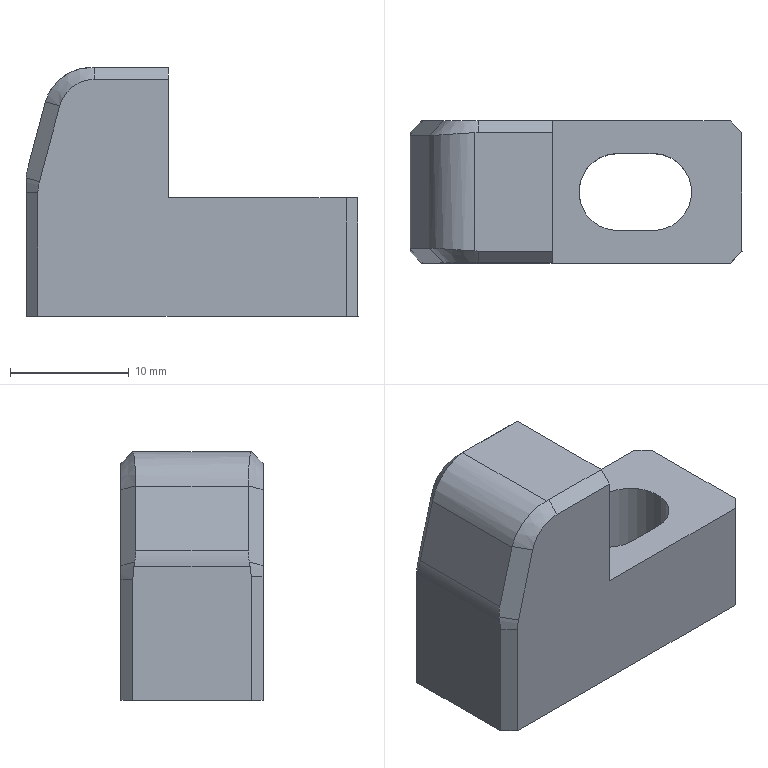Part | STEP file | gslz 2016.10.28-6_id682_x_t | 1 solid | 27 faces | box 28.004 x 12 x 21.002 mm | volume 4222 mm3 | plane 19 | cylinder 4 | cone 4 | commonest cylinder face diameters 6.5 x2 8 x1 10 x1
STEP:
#1=CARTESIAN_POINT('',(138.4,170.,84.004));
#2=VERTEX_POINT('',#1);
#3=CARTESIAN_POINT('',(138.4,180.,84.004));
#4=VERTEX_POINT('',#3);
#5=CARTESIAN_POINT('',(138.4,181.,84.004));
#6=DIRECTION('',(-0.000004439,1.,0.000000014));
#7=VECTOR('',#6,1.);
#8=LINE('',#5,#7);
#9=EDGE_CURVE('',#2,#4,#8,.T.);
#10=ORIENTED_EDGE('',*,*,#9,.T.);
#11=CARTESIAN_POINT('',(137.4,181.,84.004));
#12=VERTEX_POINT('',#11);
#13=CARTESIAN_POINT('',(126.128,192.272,84.002));
#14=DIRECTION('',(0.7071,-0.7071,0.0001154));
#15=VECTOR('',#14,1.);
#16=LINE('',#13,#15);
#17=EDGE_CURVE('',#12,#4,#16,.T.);
#18=ORIENTED_EDGE('',*,*,#17,.F.);
#19=CARTESIAN_POINT('',(122.4,181.,84.001));
#20=VERTEX_POINT('',#19);
#21=CARTESIAN_POINT('',(114.856,181.,84.));
#22=DIRECTION('',(1.,0.000004636,0.0001633));
#23=VECTOR('',#22,1.);
#24=LINE('',#21,#23);
#25=EDGE_CURVE('',#20,#12,#24,.T.);
#26=ORIENTED_EDGE('',*,*,#25,.F.);
#27=CARTESIAN_POINT('',(122.4,169.,84.001));
#28=VERTEX_POINT('',#27);
#29=CARTESIAN_POINT('',(122.4,181.,84.001));
#30=DIRECTION('',(0.000004439,-1.,-0.000000014));
#31=VECTOR('',#30,1.);
#32=LINE('',#29,#31);
#33=EDGE_CURVE('',#20,#28,#32,.T.);
#34=ORIENTED_EDGE('',*,*,#33,.T.);
#35=CARTESIAN_POINT('',(137.4,169.,84.004));
#36=VERTEX_POINT('',#35);
#37=CARTESIAN_POINT('',(114.856,169.,84.));
#38=DIRECTION('',(1.,0.000004636,0.0001633));
#39=VECTOR('',#38,1.);
#40=LINE('',#37,#39);
#41=EDGE_CURVE('',#28,#36,#40,.T.);
#42=ORIENTED_EDGE('',*,*,#41,.T.);
#43=CARTESIAN_POINT('',(138.4,170.,84.004));
#44=DIRECTION('',(-0.7071,-0.7071,-0.0001155));
#45=VECTOR('',#44,1.);
#46=LINE('',#43,#45);
#47=EDGE_CURVE('',#2,#36,#46,.T.);
#48=ORIENTED_EDGE('',*,*,#47,.F.);
#49=EDGE_LOOP('',(#10,#18,#26,#34,#42,#48));
#50=FACE_BOUND('',#49,.T.);
#51=CARTESIAN_POINT('',(127.9,178.25,84.002));
#52=VERTEX_POINT('',#51);
#53=CARTESIAN_POINT('',(127.9,171.75,84.002));
#54=VERTEX_POINT('',#53);
#55=CARTESIAN_POINT('',(127.9,175.,84.002));
#56=DIRECTION('',(-0.0001633,-0.000000015,1.));
#57=DIRECTION('',(-1.,0.,-0.0001633));
#58=AXIS2_PLACEMENT_3D('',#55,#56,#57);
#59=CIRCLE('',#58,3.25);
#60=EDGE_CURVE('',#52,#54,#59,.T.);
#61=ORIENTED_EDGE('',*,*,#60,.F.);
#62=CARTESIAN_POINT('',(130.9,178.25,84.003));
#63=VERTEX_POINT('',#62);
#64=CARTESIAN_POINT('',(130.9,178.25,84.003));
#65=DIRECTION('',(-1.,-0.000004439,-0.0001633));
#66=VECTOR('',#65,1.);
#67=LINE('',#64,#66);
#68=EDGE_CURVE('',#63,#52,#67,.T.);
#69=ORIENTED_EDGE('',*,*,#68,.F.);
#70=CARTESIAN_POINT('',(130.9,171.75,84.003));
#71=VERTEX_POINT('',#70);
#72=CARTESIAN_POINT('',(130.9,175.,84.003));
#73=DIRECTION('',(-0.0001633,-0.000000015,1.));
#74=DIRECTION('',(-1.,0.,-0.0001633));
#75=AXIS2_PLACEMENT_3D('',#72,#73,#74);
#76=CIRCLE('',#75,3.25);
#77=EDGE_CURVE('',#71,#63,#76,.T.);
#78=ORIENTED_EDGE('',*,*,#77,.F.);
#79=CARTESIAN_POINT('',(130.9,171.75,84.003));
#80=DIRECTION('',(1.,0.000004439,0.0001633));
#81=VECTOR('',#80,1.);
#82=LINE('',#79,#81);
#83=EDGE_CURVE('',#54,#71,#82,.T.);
#84=ORIENTED_EDGE('',*,*,#83,.F.);
#85=EDGE_LOOP('',(#61,#69,#78,#84));
#86=FACE_BOUND('',#85,.T.);
#87=CARTESIAN_POINT('',(114.856,181.,84.));
#88=DIRECTION('',(0.0001633,0.000000015,-1.));
#89=DIRECTION('',(-1.,-0.000004636,-0.0001633));
#90=AXIS2_PLACEMENT_3D('',#87,#88,#89);
#91=PLANE('',#90);
#92=ADVANCED_FACE('',(#50,#86),#91,.F.);
#93=CARTESIAN_POINT('',(111.402,169.,73.999));
#94=VERTEX_POINT('',#93);
#95=CARTESIAN_POINT('',(137.402,169.,74.004));
#96=VERTEX_POINT('',#95);
#97=CARTESIAN_POINT('',(114.858,169.,74.));
#98=DIRECTION('',(1.,0.000004636,0.0001633));
#99=VECTOR('',#98,1.);
#100=LINE('',#97,#99);
#101=EDGE_CURVE('',#94,#96,#100,.T.);
#102=ORIENTED_EDGE('',*,*,#101,.F.);
#103=CARTESIAN_POINT('',(110.402,170.,73.999));
#104=VERTEX_POINT('',#103);
#105=CARTESIAN_POINT('',(107.13,173.272,73.999));
#106=DIRECTION('',(0.7071,-0.7071,0.0001154));
#107=VECTOR('',#106,1.);
#108=LINE('',#105,#107);
#109=EDGE_CURVE('',#104,#94,#108,.T.);
#110=ORIENTED_EDGE('',*,*,#109,.F.);
#111=CARTESIAN_POINT('',(110.402,180.,73.999));
#112=VERTEX_POINT('',#111);
#113=CARTESIAN_POINT('',(110.401,405.866,73.999));
#114=DIRECTION('',(-0.000004439,1.,0.000000014));
#115=VECTOR('',#114,1.);
#116=LINE('',#113,#115);
#117=EDGE_CURVE('',#104,#112,#116,.T.);
#118=ORIENTED_EDGE('',*,*,#117,.T.);
#119=CARTESIAN_POINT('',(111.402,181.,73.999));
#120=VERTEX_POINT('',#119);
#121=CARTESIAN_POINT('',(113.13,182.728,74.));
#122=DIRECTION('',(-0.7071,-0.7071,-0.0001155));
#123=VECTOR('',#122,1.);
#124=LINE('',#121,#123);
#125=EDGE_CURVE('',#120,#112,#124,.T.);
#126=ORIENTED_EDGE('',*,*,#125,.F.);
#127=CARTESIAN_POINT('',(137.402,181.,74.004));
#128=VERTEX_POINT('',#127);
#129=CARTESIAN_POINT('',(114.858,181.,74.));
#130=DIRECTION('',(1.,0.000004636,0.0001633));
#131=VECTOR('',#130,1.);
#132=LINE('',#129,#131);
#133=EDGE_CURVE('',#120,#128,#132,.T.);
#134=ORIENTED_EDGE('',*,*,#133,.T.);
#135=CARTESIAN_POINT('',(138.402,180.,74.004));
#136=VERTEX_POINT('',#135);
#137=CARTESIAN_POINT('',(137.402,181.,74.004));
#138=DIRECTION('',(-0.7071,0.7071,-0.0001154));
#139=VECTOR('',#138,1.);
#140=LINE('',#137,#139);
#141=EDGE_CURVE('',#136,#128,#140,.T.);
#142=ORIENTED_EDGE('',*,*,#141,.F.);
#143=CARTESIAN_POINT('',(138.402,170.,74.004));
#144=VERTEX_POINT('',#143);
#145=CARTESIAN_POINT('',(138.402,181.,74.004));
#146=DIRECTION('',(-0.000004439,1.,0.000000014));
#147=VECTOR('',#146,1.);
#148=LINE('',#145,#147);
#149=EDGE_CURVE('',#144,#136,#148,.T.);
#150=ORIENTED_EDGE('',*,*,#149,.F.);
#151=CARTESIAN_POINT('',(132.13,163.728,74.003));
#152=DIRECTION('',(0.7071,0.7071,0.0001155));
#153=VECTOR('',#152,1.);
#154=LINE('',#151,#153);
#155=EDGE_CURVE('',#96,#144,#154,.T.);
#156=ORIENTED_EDGE('',*,*,#155,.F.);
#157=EDGE_LOOP('',(#102,#110,#118,#126,#134,#142,#150,#156));
#158=FACE_BOUND('',#157,.T.);
#159=CARTESIAN_POINT('',(130.902,178.25,74.003));
#160=VERTEX_POINT('',#159);
#161=CARTESIAN_POINT('',(130.902,171.75,74.003));
#162=VERTEX_POINT('',#161);
#163=CARTESIAN_POINT('',(130.902,175.,74.003));
#164=DIRECTION('',(0.0001633,0.000000015,-1.));
#165=DIRECTION('',(-1.,0.,-0.0001633));
#166=AXIS2_PLACEMENT_3D('',#163,#164,#165);
#167=CIRCLE('',#166,3.25);
#168=EDGE_CURVE('',#160,#162,#167,.T.);
#169=ORIENTED_EDGE('',*,*,#168,.F.);
#170=CARTESIAN_POINT('',(127.902,178.25,74.002));
#171=VERTEX_POINT('',#170);
#172=CARTESIAN_POINT('',(114.858,178.25,74.));
#173=DIRECTION('',(1.,0.000004439,0.0001633));
#174=VECTOR('',#173,1.);
#175=LINE('',#172,#174);
#176=EDGE_CURVE('',#171,#160,#175,.T.);
#177=ORIENTED_EDGE('',*,*,#176,.F.);
#178=CARTESIAN_POINT('',(127.902,171.75,74.002));
#179=VERTEX_POINT('',#178);
#180=CARTESIAN_POINT('',(127.902,175.,74.002));
#181=DIRECTION('',(-0.0001633,-0.000000015,1.));
#182=DIRECTION('',(-1.,0.,-0.0001633));
#183=AXIS2_PLACEMENT_3D('',#180,#181,#182);
#184=CIRCLE('',#183,3.25);
#185=EDGE_CURVE('',#171,#179,#184,.T.);
#186=ORIENTED_EDGE('',*,*,#185,.T.);
#187=CARTESIAN_POINT('',(114.858,171.75,74.));
#188=DIRECTION('',(-1.,-0.000004439,-0.0001633));
#189=VECTOR('',#188,1.);
#190=LINE('',#187,#189);
#191=EDGE_CURVE('',#162,#179,#190,.T.);
#192=ORIENTED_EDGE('',*,*,#191,.F.);
#193=EDGE_LOOP('',(#169,#177,#186,#192));
#194=FACE_BOUND('',#193,.T.);
#195=CARTESIAN_POINT('',(114.858,181.,74.));
#196=DIRECTION('',(0.0001633,0.000000015,-1.));
#197=DIRECTION('',(-1.,-0.000004636,-0.0001633));
#198=AXIS2_PLACEMENT_3D('',#195,#196,#197);
#199=PLANE('',#198);
#200=ADVANCED_FACE('',(#158,#194),#199,.T.);
#201=ORIENTED_EDGE('',*,*,#149,.T.);
#202=CARTESIAN_POINT('',(138.399,180.,91.479));
#203=DIRECTION('',(0.0001633,0.000000015,-1.));
#204=VECTOR('',#203,1.);
#205=LINE('',#202,#204);
#206=EDGE_CURVE('',#4,#136,#205,.T.);
#207=ORIENTED_EDGE('',*,*,#206,.F.);
#208=ORIENTED_EDGE('',*,*,#9,.F.);
#209=CARTESIAN_POINT('',(138.4,170.,84.004));
#210=DIRECTION('',(-0.0001633,-0.000000015,1.));
#211=VECTOR('',#210,1.);
#212=LINE('',#209,#211);
#213=EDGE_CURVE('',#144,#2,#212,.T.);
#214=ORIENTED_EDGE('',*,*,#213,.F.);
#215=EDGE_LOOP('',(#201,#207,#208,#214));
#216=FACE_OUTER_BOUND('',#215,.T.);
#217=CARTESIAN_POINT('',(138.398,405.866,91.479));
#218=DIRECTION('',(-1.,-0.000004439,-0.0001633));
#219=DIRECTION('',(-0.00001298,0.9986,0.05234));
#220=AXIS2_PLACEMENT_3D('',#217,#218,#219);
#221=PLANE('',#220);
#222=ADVANCED_FACE('',(#216),#221,.F.);
#223=ORIENTED_EDGE('',*,*,#117,.F.);
#224=CARTESIAN_POINT('',(110.399,170.001,84.462));
#225=VERTEX_POINT('',#224);
#226=CARTESIAN_POINT('',(110.396,170.002,91.507));
#227=DIRECTION('',(0.0003054,-0.0001421,-1.));
#228=VECTOR('',#227,1.);
#229=LINE('',#226,#228);
#230=EDGE_CURVE('',#225,#104,#229,.T.);
#231=ORIENTED_EDGE('',*,*,#230,.F.);
#232=CARTESIAN_POINT('',(110.398,170.099,85.339));
#233=VERTEX_POINT('',#232);
#234=CARTESIAN_POINT('',(110.398,170.099,85.339));
#235=CARTESIAN_POINT('',(110.398,170.042,85.05));
#236=CARTESIAN_POINT('',(110.398,170.009,84.756));
#237=CARTESIAN_POINT('',(110.399,170.001,84.462));
#238=B_SPLINE_CURVE_WITH_KNOTS('',3,(#234,#235,#236,#237),.UNSPECIFIED.,.F.,.F.,(4,4),(0.,1.),.UNSPECIFIED.);
#239=EDGE_CURVE('',#233,#225,#238,.T.);
#240=ORIENTED_EDGE('',*,*,#239,.F.);
#241=CARTESIAN_POINT('',(110.398,179.901,85.339));
#242=VERTEX_POINT('',#241);
#243=CARTESIAN_POINT('',(110.397,405.866,85.339));
#244=DIRECTION('',(0.000004439,-1.,-0.000000014));
#245=VECTOR('',#244,1.);
#246=LINE('',#243,#245);
#247=EDGE_CURVE('',#242,#233,#246,.T.);
#248=ORIENTED_EDGE('',*,*,#247,.F.);
#249=CARTESIAN_POINT('',(110.399,179.998,84.22));
#250=VERTEX_POINT('',#249);
#251=CARTESIAN_POINT('',(110.398,179.901,85.339));
#252=CARTESIAN_POINT('',(110.398,179.973,84.972));
#253=CARTESIAN_POINT('',(110.398,180.007,84.594));
#254=CARTESIAN_POINT('',(110.399,179.998,84.22));
#255=B_SPLINE_CURVE_WITH_KNOTS('',3,(#251,#252,#253,#254),.UNSPECIFIED.,.F.,.F.,(4,4),(0.,1.),.UNSPECIFIED.);
#256=EDGE_CURVE('',#242,#250,#255,.T.);
#257=ORIENTED_EDGE('',*,*,#256,.T.);
#258=CARTESIAN_POINT('',(110.396,179.997,91.474));
#259=DIRECTION('',(-0.0003054,-0.0001421,1.));
#260=VECTOR('',#259,1.);
#261=LINE('',#258,#260);
#262=EDGE_CURVE('',#112,#250,#261,.T.);
#263=ORIENTED_EDGE('',*,*,#262,.F.);
#264=EDGE_LOOP('',(#223,#231,#240,#248,#257,#263));
#265=FACE_OUTER_BOUND('',#264,.T.);
#266=CARTESIAN_POINT('',(110.395,405.866,91.474));
#267=DIRECTION('',(-1.,-0.000004439,-0.0003054));
#268=DIRECTION('',(-0.00002041,0.9986,0.05234));
#269=AXIS2_PLACEMENT_3D('',#266,#267,#268);
#270=PLANE('',#269);
#271=ADVANCED_FACE('',(#265),#270,.T.);
#272=ORIENTED_EDGE('',*,*,#133,.F.);
#273=CARTESIAN_POINT('',(111.4,181.,84.233));
#274=VERTEX_POINT('',#273);
#275=CARTESIAN_POINT('',(111.402,181.,73.999));
#276=DIRECTION('',(0.0001633,0.000000015,-1.));
#277=VECTOR('',#276,1.);
#278=LINE('',#275,#277);
#279=EDGE_CURVE('',#274,#120,#278,.T.);
#280=ORIENTED_EDGE('',*,*,#279,.F.);
#281=CARTESIAN_POINT('',(111.535,181.,85.376));
#282=VERTEX_POINT('',#281);
#283=CARTESIAN_POINT('',(115.399,181.,84.342));
#284=DIRECTION('',(0.000004636,-1.,-0.000000014));
#285=DIRECTION('',(1.,0.000004636,0.0001633));
#286=AXIS2_PLACEMENT_3D('',#283,#284,#285);
#287=CIRCLE('',#286,4.);
#288=EDGE_CURVE('',#282,#274,#287,.T.);
#289=ORIENTED_EDGE('',*,*,#288,.F.);
#290=CARTESIAN_POINT('',(113.248,181.,91.776));
#291=VERTEX_POINT('',#290);
#292=CARTESIAN_POINT('',(106.666,181.,67.194));
#293=DIRECTION('',(-0.2587,-0.000001186,-0.966));
#294=VECTOR('',#293,1.);
#295=LINE('',#292,#294);
#296=EDGE_CURVE('',#291,#282,#295,.T.);
#297=ORIENTED_EDGE('',*,*,#296,.F.);
#298=CARTESIAN_POINT('',(116.146,181.,94.));
#299=VERTEX_POINT('',#298);
#300=CARTESIAN_POINT('',(116.146,181.,91.));
#301=DIRECTION('',(0.000004636,-1.,-0.000000014));
#302=DIRECTION('',(1.,0.000004636,0.0001633));
#303=AXIS2_PLACEMENT_3D('',#300,#301,#302);
#304=CIRCLE('',#303,3.);
#305=EDGE_CURVE('',#299,#291,#304,.T.);
#306=ORIENTED_EDGE('',*,*,#305,.F.);
#307=CARTESIAN_POINT('',(122.398,181.,94.001));
#308=VERTEX_POINT('',#307);
#309=CARTESIAN_POINT('',(116.146,181.,94.));
#310=DIRECTION('',(-1.,-0.000004636,-0.0001633));
#311=VECTOR('',#310,1.);
#312=LINE('',#309,#311);
#313=EDGE_CURVE('',#308,#299,#312,.T.);
#314=ORIENTED_EDGE('',*,*,#313,.F.);
#315=CARTESIAN_POINT('',(122.4,181.,84.001));
#316=DIRECTION('',(-0.0001633,-0.000000015,1.));
#317=VECTOR('',#316,1.);
#318=LINE('',#315,#317);
#319=EDGE_CURVE('',#20,#308,#318,.T.);
#320=ORIENTED_EDGE('',*,*,#319,.F.);
#321=ORIENTED_EDGE('',*,*,#25,.T.);
#322=CARTESIAN_POINT('',(137.402,181.,74.004));
#323=DIRECTION('',(-0.0001633,-0.000000015,1.));
#324=VECTOR('',#323,1.);
#325=LINE('',#322,#324);
#326=EDGE_CURVE('',#128,#12,#325,.T.);
#327=ORIENTED_EDGE('',*,*,#326,.F.);
#328=EDGE_LOOP('',(#272,#280,#289,#297,#306,#314,#320,#321,#327));
#329=FACE_OUTER_BOUND('',#328,.T.);
#330=CARTESIAN_POINT('',(114.858,181.,74.));
#331=DIRECTION('',(-0.000004636,1.,0.000000014));
#332=DIRECTION('',(-1.,-0.000004636,-0.0001633));
#333=AXIS2_PLACEMENT_3D('',#330,#331,#332);
#334=PLANE('',#333);
#335=ADVANCED_FACE('',(#329),#334,.T.);
#336=ORIENTED_EDGE('',*,*,#41,.F.);
#337=CARTESIAN_POINT('',(122.399,169.,94.001));
#338=VERTEX_POINT('',#337);
#339=CARTESIAN_POINT('',(122.4,169.,84.001));
#340=DIRECTION('',(-0.0001633,-0.000000015,1.));
#341=VECTOR('',#340,1.);
#342=LINE('',#339,#341);
#343=EDGE_CURVE('',#28,#338,#342,.T.);
#344=ORIENTED_EDGE('',*,*,#343,.T.);
#345=CARTESIAN_POINT('',(116.146,169.,94.));
#346=VERTEX_POINT('',#345);
#347=CARTESIAN_POINT('',(114.853,169.,94.));
#348=DIRECTION('',(1.,0.000004636,0.0001633));
#349=VECTOR('',#348,1.);
#350=LINE('',#347,#349);
#351=EDGE_CURVE('',#346,#338,#350,.T.);
#352=ORIENTED_EDGE('',*,*,#351,.F.);
#353=CARTESIAN_POINT('',(113.248,169.,91.776));
#354=VERTEX_POINT('',#353);
#355=CARTESIAN_POINT('',(116.146,169.,91.));
#356=DIRECTION('',(-0.000004636,1.,0.000000014));
#357=DIRECTION('',(1.,0.000004636,0.0001633));
#358=AXIS2_PLACEMENT_3D('',#355,#356,#357);
#359=CIRCLE('',#358,3.);
#360=EDGE_CURVE('',#354,#346,#359,.T.);
#361=ORIENTED_EDGE('',*,*,#360,.F.);
#362=CARTESIAN_POINT('',(111.535,169.,85.376));
#363=VERTEX_POINT('',#362);
#364=CARTESIAN_POINT('',(113.248,169.,91.776));
#365=DIRECTION('',(0.2587,0.000001186,0.966));
#366=VECTOR('',#365,1.);
#367=LINE('',#364,#366);
#368=EDGE_CURVE('',#363,#354,#367,.T.);
#369=ORIENTED_EDGE('',*,*,#368,.F.);
#370=CARTESIAN_POINT('',(111.4,169.,84.45));
#371=VERTEX_POINT('',#370);
#372=CARTESIAN_POINT('',(115.399,169.,84.342));
#373=DIRECTION('',(-0.000004636,1.,0.000000014));
#374=DIRECTION('',(1.,0.000004636,0.0001633));
#375=AXIS2_PLACEMENT_3D('',#372,#373,#374);
#376=CIRCLE('',#375,4.);
#377=EDGE_CURVE('',#371,#363,#376,.T.);
#378=ORIENTED_EDGE('',*,*,#377,.F.);
#379=CARTESIAN_POINT('',(111.399,169.,93.341));
#380=DIRECTION('',(-0.0001633,-0.000000015,1.));
#381=VECTOR('',#380,1.);
#382=LINE('',#379,#381);
#383=EDGE_CURVE('',#94,#371,#382,.T.);
#384=ORIENTED_EDGE('',*,*,#383,.F.);
#385=ORIENTED_EDGE('',*,*,#101,.T.);
#386=CARTESIAN_POINT('',(137.402,169.,74.004));
#387=DIRECTION('',(0.0001633,0.000000015,-1.));
#388=VECTOR('',#387,1.);
#389=LINE('',#386,#388);
#390=EDGE_CURVE('',#36,#96,#389,.T.);
#391=ORIENTED_EDGE('',*,*,#390,.F.);
#392=EDGE_LOOP('',(#336,#344,#352,#361,#369,#378,#384,#385,#391));
#393=FACE_OUTER_BOUND('',#392,.T.);
#394=CARTESIAN_POINT('',(114.858,169.,74.));
#395=DIRECTION('',(-0.000004636,1.,0.000000014));
#396=DIRECTION('',(-1.,-0.000004636,-0.0001633));
#397=AXIS2_PLACEMENT_3D('',#394,#395,#396);
#398=PLANE('',#397);
#399=ADVANCED_FACE('',(#393),#398,.F.);
#400=CARTESIAN_POINT('',(122.398,180.,95.001));
#401=VERTEX_POINT('',#400);
#402=CARTESIAN_POINT('',(122.398,170.,95.001));
#403=VERTEX_POINT('',#402);
#404=CARTESIAN_POINT('',(122.398,181.,95.001));
#405=DIRECTION('',(0.000004439,-1.,-0.000000014));
#406=VECTOR('',#405,1.);
#407=LINE('',#404,#406);
#408=EDGE_CURVE('',#401,#403,#407,.T.);
#409=ORIENTED_EDGE('',*,*,#408,.T.);
#410=CARTESIAN_POINT('',(122.398,170.,95.001));
#411=DIRECTION('',(-0.0001186,0.7071,0.7071));
#412=VECTOR('',#411,1.);
#413=LINE('',#410,#412);
#414=EDGE_CURVE('',#338,#403,#413,.T.);
#415=ORIENTED_EDGE('',*,*,#414,.F.);
#416=ORIENTED_EDGE('',*,*,#343,.F.);
#417=ORIENTED_EDGE('',*,*,#33,.F.);
#418=ORIENTED_EDGE('',*,*,#319,.T.);
#419=CARTESIAN_POINT('',(122.399,186.,89.001));
#420=DIRECTION('',(0.0001123,0.7071,-0.7071));
#421=VECTOR('',#420,1.);
#422=LINE('',#419,#421);
#423=EDGE_CURVE('',#401,#308,#422,.T.);
#424=ORIENTED_EDGE('',*,*,#423,.F.);
#425=EDGE_LOOP('',(#409,#415,#416,#417,#418,#424));
#426=FACE_OUTER_BOUND('',#425,.T.);
#427=CARTESIAN_POINT('',(122.4,181.,84.001));
#428=DIRECTION('',(1.,0.000004439,0.0001633));
#429=DIRECTION('',(-0.000004439,1.,0.000000014));
#430=AXIS2_PLACEMENT_3D('',#427,#428,#429);
#431=PLANE('',#430);
#432=ADVANCED_FACE('',(#426),#431,.T.);
#433=CARTESIAN_POINT('',(110.568,170.259,86.634));
#434=VERTEX_POINT('',#433);
#435=CARTESIAN_POINT('',(110.568,179.741,86.634));
#436=VERTEX_POINT('',#435);
#437=CARTESIAN_POINT('',(110.568,181.,86.634));
#438=DIRECTION('',(-0.000004439,1.,0.000000014));
#439=VECTOR('',#438,1.);
#440=LINE('',#437,#439);
#441=EDGE_CURVE('',#434,#436,#440,.T.);
#442=ORIENTED_EDGE('',*,*,#441,.F.);
#443=CARTESIAN_POINT('',(112.015,170.259,92.035));
#444=VERTEX_POINT('',#443);
#445=CARTESIAN_POINT('',(112.897,170.259,95.33));
#446=DIRECTION('',(-0.2587,-0.000001186,-0.966));
#447=VECTOR('',#446,1.);
#448=LINE('',#445,#447);
#449=EDGE_CURVE('',#444,#434,#448,.T.);
#450=ORIENTED_EDGE('',*,*,#449,.F.);
#451=CARTESIAN_POINT('',(112.015,179.741,92.035));
#452=VERTEX_POINT('',#451);
#453=CARTESIAN_POINT('',(112.015,181.,92.035));
#454=DIRECTION('',(0.000004439,-1.,-0.000000014));
#455=VECTOR('',#454,1.);
#456=LINE('',#453,#455);
#457=EDGE_CURVE('',#452,#444,#456,.T.);
#458=ORIENTED_EDGE('',*,*,#457,.F.);
#459=CARTESIAN_POINT('',(105.45,179.741,67.519));
#460=DIRECTION('',(0.2587,0.000001186,0.966));
#461=VECTOR('',#460,1.);
#462=LINE('',#459,#461);
#463=EDGE_CURVE('',#436,#452,#462,.T.);
#464=ORIENTED_EDGE('',*,*,#463,.F.);
#465=EDGE_LOOP('',(#442,#450,#458,#464));
#466=FACE_OUTER_BOUND('',#465,.T.);
#467=CARTESIAN_POINT('',(112.897,181.,95.33));
#468=DIRECTION('',(-0.966,-0.000004291,0.2587));
#469=DIRECTION('',(0.000004439,-1.,-0.000000014));
#470=AXIS2_PLACEMENT_3D('',#467,#468,#469);
#471=PLANE('',#470);
#472=ADVANCED_FACE('',(#466),#471,.T.);
#473=CARTESIAN_POINT('',(115.878,170.009,95.));
#474=VERTEX_POINT('',#473);
#475=CARTESIAN_POINT('',(115.878,179.991,95.));
#476=VERTEX_POINT('',#475);
#477=CARTESIAN_POINT('',(115.878,181.,95.));
#478=DIRECTION('',(-0.000004439,1.,0.000000014));
#479=VECTOR('',#478,1.);
#480=LINE('',#477,#479);
#481=EDGE_CURVE('',#474,#476,#480,.T.);
#482=ORIENTED_EDGE('',*,*,#481,.F.);
#483=CARTESIAN_POINT('',(116.146,170.,95.));
#484=VERTEX_POINT('',#483);
#485=CARTESIAN_POINT('',(115.878,170.009,95.));
#486=CARTESIAN_POINT('',(115.967,170.003,95.));
#487=CARTESIAN_POINT('',(116.056,170.,95.));
#488=CARTESIAN_POINT('',(116.146,170.,95.));
#489=B_SPLINE_CURVE_WITH_KNOTS('',3,(#485,#486,#487,#488),.UNSPECIFIED.,.F.,.F.,(4,4),(0.,1.),.UNSPECIFIED.);
#490=EDGE_CURVE('',#474,#484,#489,.T.);
#491=ORIENTED_EDGE('',*,*,#490,.T.);
#492=CARTESIAN_POINT('',(110.397,170.,94.999));
#493=DIRECTION('',(-1.,-0.000004636,-0.0001633));
#494=VECTOR('',#493,1.);
#495=LINE('',#492,#494);
#496=EDGE_CURVE('',#403,#484,#495,.T.);
#497=ORIENTED_EDGE('',*,*,#496,.F.);
#498=ORIENTED_EDGE('',*,*,#408,.F.);
#499=CARTESIAN_POINT('',(116.146,180.,95.));
#500=VERTEX_POINT('',#499);
#501=CARTESIAN_POINT('',(122.397,180.,95.001));
#502=DIRECTION('',(1.,0.000004636,0.0001633));
#503=VECTOR('',#502,1.);
#504=LINE('',#501,#503);
#505=EDGE_CURVE('',#500,#401,#504,.T.);
#506=ORIENTED_EDGE('',*,*,#505,.F.);
#507=CARTESIAN_POINT('',(115.878,179.991,95.));
#508=CARTESIAN_POINT('',(115.967,179.997,95.));
#509=CARTESIAN_POINT('',(116.056,180.,95.));
#510=CARTESIAN_POINT('',(116.146,180.,95.));
#511=B_SPLINE_CURVE_WITH_KNOTS('',3,(#507,#508,#509,#510),.UNSPECIFIED.,.F.,.F.,(4,4),(0.,1.),.UNSPECIFIED.);
#512=EDGE_CURVE('',#476,#500,#511,.T.);
#513=ORIENTED_EDGE('',*,*,#512,.F.);
#514=EDGE_LOOP('',(#482,#491,#497,#498,#506,#513));
#515=FACE_OUTER_BOUND('',#514,.T.);
#516=CARTESIAN_POINT('',(110.397,181.,94.999));
#517=DIRECTION('',(0.0001633,0.000000015,-1.));
#518=DIRECTION('',(-0.000004439,1.,0.000000014));
#519=AXIS2_PLACEMENT_3D('',#516,#517,#518);
#520=PLANE('',#519);
#521=ADVANCED_FACE('',(#515),#520,.F.);
#522=ORIENTED_EDGE('',*,*,#457,.T.);
#523=CARTESIAN_POINT('',(112.033,170.258,92.102));
#524=VERTEX_POINT('',#523);
#525=CARTESIAN_POINT('',(115.879,166.259,91.));
#526=DIRECTION('',(-0.683,-0.7071,0.1829));
#527=DIRECTION('',(-0.683,0.7071,0.1829));
#528=AXIS2_PLACEMENT_3D('',#525,#526,#527);
#529=ELLIPSE('',#528,5.657,4.);
#530=EDGE_CURVE('',#524,#444,#529,.T.);
#531=ORIENTED_EDGE('',*,*,#530,.F.);
#532=CARTESIAN_POINT('',(115.878,170.009,95.));
#533=CARTESIAN_POINT('',(115.483,170.035,95.));
#534=CARTESIAN_POINT('',(115.084,170.062,94.94));
#535=CARTESIAN_POINT('',(114.706,170.086,94.824));
#536=CARTESIAN_POINT('',(114.277,170.114,94.693));
#537=CARTESIAN_POINT('',(113.865,170.141,94.485));
#538=CARTESIAN_POINT('',(113.504,170.164,94.219));
#539=CARTESIAN_POINT('',(113.143,170.188,93.953));
#540=CARTESIAN_POINT('',(112.823,170.208,93.62));
#541=CARTESIAN_POINT('',(112.571,170.224,93.249));
#542=CARTESIAN_POINT('',(112.333,170.239,92.9));
#543=CARTESIAN_POINT('',(112.15,170.251,92.508));
#544=CARTESIAN_POINT('',(112.033,170.258,92.102));
#545=B_SPLINE_CURVE_WITH_KNOTS('',3,(#532,#533,#534,#535,#536,#537,#538,#539,#540,#541,#542,#543,#544),.UNSPECIFIED.,.F.,.F.,(4,3,3,3,4),(0.,0.23,0.4922,0.754,1.),.UNSPECIFIED.);
#546=EDGE_CURVE('',#474,#524,#545,.T.);
#547=ORIENTED_EDGE('',*,*,#546,.F.);
#548=ORIENTED_EDGE('',*,*,#481,.T.);
#549=CARTESIAN_POINT('',(112.033,179.742,92.102));
#550=VERTEX_POINT('',#549);
#551=CARTESIAN_POINT('',(112.033,179.742,92.102));
#552=CARTESIAN_POINT('',(112.149,179.749,92.506));
#553=CARTESIAN_POINT('',(112.332,179.761,92.897));
#554=CARTESIAN_POINT('',(112.568,179.776,93.245));
#555=CARTESIAN_POINT('',(112.819,179.792,93.615));
#556=CARTESIAN_POINT('',(113.137,179.812,93.947));
#557=CARTESIAN_POINT('',(113.496,179.835,94.213));
#558=CARTESIAN_POINT('',(113.855,179.858,94.479));
#559=CARTESIAN_POINT('',(114.265,179.885,94.688));
#560=CARTESIAN_POINT('',(114.692,179.912,94.82));
#561=CARTESIAN_POINT('',(115.074,179.938,94.939));
#562=CARTESIAN_POINT('',(115.478,179.964,95.));
#563=CARTESIAN_POINT('',(115.878,179.991,95.));
#564=B_SPLINE_CURVE_WITH_KNOTS('',3,(#551,#552,#553,#554,#555,#556,#557,#558,#559,#560,#561,#562,#563),.UNSPECIFIED.,.F.,.F.,(4,3,3,3,4),(0.,0.2451,0.5059,0.7671,1.),.UNSPECIFIED.);
#565=EDGE_CURVE('',#550,#476,#564,.T.);
#566=ORIENTED_EDGE('',*,*,#565,.F.);
#567=CARTESIAN_POINT('',(115.878,183.741,91.));
#568=DIRECTION('',(0.683,-0.7071,-0.1829));
#569=DIRECTION('',(0.683,0.7071,-0.1829));
#570=AXIS2_PLACEMENT_3D('',#567,#568,#569);
#571=ELLIPSE('',#570,5.657,4.);
#572=EDGE_CURVE('',#550,#452,#571,.T.);
#573=ORIENTED_EDGE('',*,*,#572,.T.);
#574=EDGE_LOOP('',(#522,#531,#547,#548,#566,#573));
#575=FACE_OUTER_BOUND('',#574,.T.);
#576=CARTESIAN_POINT('',(115.878,181.,91.));
#577=DIRECTION('',(-0.000004439,1.,0.000000014));
#578=DIRECTION('',(-1.,-0.000004439,0.));
#579=AXIS2_PLACEMENT_3D('',#576,#577,#578);
#580=CYLINDRICAL_SURFACE('',#579,4.);
#581=ADVANCED_FACE('',(#575),#580,.T.);
#582=ORIENTED_EDGE('',*,*,#60,.T.);
#583=CARTESIAN_POINT('',(127.902,171.75,73.002));
#584=DIRECTION('',(-0.0001633,-0.000000015,1.));
#585=VECTOR('',#584,1.);
#586=LINE('',#583,#585);
#587=EDGE_CURVE('',#179,#54,#586,.T.);
#588=ORIENTED_EDGE('',*,*,#587,.F.);
#589=ORIENTED_EDGE('',*,*,#185,.F.);
#590=CARTESIAN_POINT('',(127.902,178.25,74.002));
#591=DIRECTION('',(-0.0001633,-0.000000015,1.));
#592=VECTOR('',#591,1.);
#593=LINE('',#590,#592);
#594=EDGE_CURVE('',#171,#52,#593,.T.);
#595=ORIENTED_EDGE('',*,*,#594,.T.);
#596=EDGE_LOOP('',(#582,#588,#589,#595));
#597=FACE_OUTER_BOUND('',#596,.T.);
#598=CARTESIAN_POINT('',(127.902,175.,73.002));
#599=DIRECTION('',(0.0001633,0.000000015,-1.));
#600=DIRECTION('',(-1.,0.,-0.0001633));
#601=AXIS2_PLACEMENT_3D('',#598,#599,#600);
#602=CYLINDRICAL_SURFACE('',#601,3.25);
#603=ADVANCED_FACE('',(#597),#602,.F.);
#604=ORIENTED_EDGE('',*,*,#247,.T.);
#605=CARTESIAN_POINT('',(110.41,170.165,85.678));
#606=VERTEX_POINT('',#605);
#607=CARTESIAN_POINT('',(110.41,170.165,85.678));
#608=CARTESIAN_POINT('',(110.402,170.143,85.565));
#609=CARTESIAN_POINT('',(110.398,170.121,85.452));
#610=CARTESIAN_POINT('',(110.398,170.099,85.339));
#611=B_SPLINE_CURVE_WITH_KNOTS('',3,(#607,#608,#609,#610),.UNSPECIFIED.,.F.,.F.,(4,4),(0.,1.),.UNSPECIFIED.);
#612=EDGE_CURVE('',#606,#233,#611,.T.);
#613=ORIENTED_EDGE('',*,*,#612,.F.);
#614=CARTESIAN_POINT('',(115.398,165.259,85.341));
#615=DIRECTION('',(0.683,0.7071,-0.1829));
#616=DIRECTION('',(0.683,-0.7071,-0.1829));
#617=AXIS2_PLACEMENT_3D('',#614,#615,#616);
#618=ELLIPSE('',#617,7.071,5.);
#619=EDGE_CURVE('',#606,#434,#618,.T.);
#620=ORIENTED_EDGE('',*,*,#619,.T.);
#621=ORIENTED_EDGE('',*,*,#441,.T.);
#622=CARTESIAN_POINT('',(110.41,179.835,85.678));
#623=VERTEX_POINT('',#622);
#624=CARTESIAN_POINT('',(115.398,184.741,85.341));
#625=DIRECTION('',(-0.683,0.7071,0.1829));
#626=DIRECTION('',(-0.683,-0.7071,0.1829));
#627=AXIS2_PLACEMENT_3D('',#624,#625,#626);
#628=ELLIPSE('',#627,7.071,5.);
#629=EDGE_CURVE('',#623,#436,#628,.T.);
#630=ORIENTED_EDGE('',*,*,#629,.F.);
#631=CARTESIAN_POINT('',(110.398,179.901,85.339));
#632=CARTESIAN_POINT('',(110.398,179.879,85.452));
#633=CARTESIAN_POINT('',(110.402,179.857,85.565));
#634=CARTESIAN_POINT('',(110.41,179.835,85.678));
#635=B_SPLINE_CURVE_WITH_KNOTS('',3,(#631,#632,#633,#634),.UNSPECIFIED.,.F.,.F.,(4,4),(0.,1.),.UNSPECIFIED.);
#636=EDGE_CURVE('',#242,#623,#635,.T.);
#637=ORIENTED_EDGE('',*,*,#636,.F.);
#638=EDGE_LOOP('',(#604,#613,#620,#621,#630,#637));
#639=FACE_OUTER_BOUND('',#638,.T.);
#640=CARTESIAN_POINT('',(115.397,405.866,85.341));
#641=DIRECTION('',(0.000004439,-1.,-0.000000014));
#642=DIRECTION('',(1.,0.000004439,0.));
#643=AXIS2_PLACEMENT_3D('',#640,#641,#642);
#644=CYLINDRICAL_SURFACE('',#643,5.);
#645=ADVANCED_FACE('',(#639),#644,.T.);
#646=ORIENTED_EDGE('',*,*,#125,.T.);
#647=ORIENTED_EDGE('',*,*,#262,.T.);
#648=CARTESIAN_POINT('',(110.399,179.998,84.22));
#649=CARTESIAN_POINT('',(110.732,180.332,84.224));
#650=CARTESIAN_POINT('',(111.066,180.666,84.228));
#651=CARTESIAN_POINT('',(111.4,181.,84.233));
#652=B_SPLINE_CURVE_WITH_KNOTS('',3,(#648,#649,#650,#651),.UNSPECIFIED.,.F.,.F.,(4,4),(0.,1.),.UNSPECIFIED.);
#653=EDGE_CURVE('',#250,#274,#652,.T.);
#654=ORIENTED_EDGE('',*,*,#653,.T.);
#655=ORIENTED_EDGE('',*,*,#279,.T.);
#656=EDGE_LOOP('',(#646,#647,#654,#655));
#657=FACE_OUTER_BOUND('',#656,.T.);
#658=CARTESIAN_POINT('',(110.399,180.,91.474));
#659=DIRECTION('',(0.7071,-0.7071,0.0001154));
#660=DIRECTION('',(0.0001633,0.000000015,-1.));
#661=AXIS2_PLACEMENT_3D('',#658,#659,#660);
#662=PLANE('',#661);
#663=ADVANCED_FACE('',(#657),#662,.F.);
#664=ORIENTED_EDGE('',*,*,#653,.F.);
#665=ORIENTED_EDGE('',*,*,#256,.F.);
#666=ORIENTED_EDGE('',*,*,#636,.T.);
#667=CARTESIAN_POINT('',(110.569,180.,85.635));
#668=DIRECTION('',(0.683,0.7071,-0.1829));
#669=VECTOR('',#668,1.);
#670=LINE('',#667,#669);
#671=EDGE_CURVE('',#623,#282,#670,.T.);
#672=ORIENTED_EDGE('',*,*,#671,.T.);
#673=ORIENTED_EDGE('',*,*,#288,.T.);
#674=EDGE_LOOP('',(#664,#665,#666,#672,#673));
#675=FACE_OUTER_BOUND('',#674,.T.);
#676=CARTESIAN_POINT('',(115.399,181.,84.342));
#677=DIRECTION('',(0.000004439,-1.,-0.000000014));
#678=DIRECTION('',(-1.,-0.000004439,-0.0001633));
#679=AXIS2_PLACEMENT_3D('',#676,#677,#678);
#680=CONICAL_SURFACE('',#679,4.,45.);
#681=ADVANCED_FACE('',(#675),#680,.T.);
#682=ORIENTED_EDGE('',*,*,#671,.F.);
#683=ORIENTED_EDGE('',*,*,#629,.T.);
#684=ORIENTED_EDGE('',*,*,#463,.T.);
#685=ORIENTED_EDGE('',*,*,#572,.F.);
#686=CARTESIAN_POINT('',(112.282,180.,92.035));
#687=DIRECTION('',(0.683,0.7071,-0.1829));
#688=VECTOR('',#687,1.);
#689=LINE('',#686,#688);
#690=EDGE_CURVE('',#550,#291,#689,.T.);
#691=ORIENTED_EDGE('',*,*,#690,.T.);
#692=ORIENTED_EDGE('',*,*,#296,.T.);
#693=EDGE_LOOP('',(#682,#683,#684,#685,#691,#692));
#694=FACE_OUTER_BOUND('',#693,.T.);
#695=CARTESIAN_POINT('',(106.666,181.,67.194));
#696=DIRECTION('',(0.683,-0.7071,-0.1829));
#697=DIRECTION('',(0.2587,0.000001186,0.966));
#698=AXIS2_PLACEMENT_3D('',#695,#696,#697);
#699=PLANE('',#698);
#700=ADVANCED_FACE('',(#694),#699,.F.);
#701=ORIENTED_EDGE('',*,*,#690,.F.);
#702=ORIENTED_EDGE('',*,*,#565,.T.);
#703=ORIENTED_EDGE('',*,*,#512,.T.);
#704=CARTESIAN_POINT('',(116.146,180.,95.));
#705=DIRECTION('',(0.0001122,0.7071,-0.7071));
#706=VECTOR('',#705,1.);
#707=LINE('',#704,#706);
#708=EDGE_CURVE('',#500,#299,#707,.T.);
#709=ORIENTED_EDGE('',*,*,#708,.T.);
#710=ORIENTED_EDGE('',*,*,#305,.T.);
#711=EDGE_LOOP('',(#701,#702,#703,#709,#710));
#712=FACE_OUTER_BOUND('',#711,.T.);
#713=CARTESIAN_POINT('',(116.146,181.,91.));
#714=DIRECTION('',(0.000004439,-1.,-0.000000014));
#715=DIRECTION('',(-1.,-0.000004439,-0.0001633));
#716=AXIS2_PLACEMENT_3D('',#713,#714,#715);
#717=CONICAL_SURFACE('',#716,3.,45.);
#718=ADVANCED_FACE('',(#712),#717,.T.);
#719=ORIENTED_EDGE('',*,*,#423,.T.);
#720=ORIENTED_EDGE('',*,*,#313,.T.);
#721=ORIENTED_EDGE('',*,*,#708,.F.);
#722=ORIENTED_EDGE('',*,*,#505,.T.);
#723=EDGE_LOOP('',(#719,#720,#721,#722));
#724=FACE_OUTER_BOUND('',#723,.T.);
#725=CARTESIAN_POINT('',(114.853,181.,94.));
#726=DIRECTION('',(-0.0001187,0.7071,0.7071));
#727=DIRECTION('',(-1.,-0.000004636,-0.0001633));
#728=AXIS2_PLACEMENT_3D('',#725,#726,#727);
#729=PLANE('',#728);
#730=ADVANCED_FACE('',(#724),#729,.T.);
#731=ORIENTED_EDGE('',*,*,#414,.T.);
#732=ORIENTED_EDGE('',*,*,#496,.T.);
#733=CARTESIAN_POINT('',(116.146,170.,95.));
#734=DIRECTION('',(0.0001187,-0.7071,-0.7071));
#735=VECTOR('',#734,1.);
#736=LINE('',#733,#735);
#737=EDGE_CURVE('',#484,#346,#736,.T.);
#738=ORIENTED_EDGE('',*,*,#737,.T.);
#739=ORIENTED_EDGE('',*,*,#351,.T.);
#740=EDGE_LOOP('',(#731,#732,#738,#739));
#741=FACE_OUTER_BOUND('',#740,.T.);
#742=CARTESIAN_POINT('',(110.397,170.,94.999));
#743=DIRECTION('',(0.0001122,0.7071,-0.7071));
#744=DIRECTION('',(0.,0.7071,0.7071));
#745=AXIS2_PLACEMENT_3D('',#742,#743,#744);
#746=PLANE('',#745);
#747=ADVANCED_FACE('',(#741),#746,.F.);
#748=ORIENTED_EDGE('',*,*,#737,.F.);
#749=ORIENTED_EDGE('',*,*,#490,.F.);
#750=ORIENTED_EDGE('',*,*,#546,.T.);
#751=CARTESIAN_POINT('',(112.282,170.,92.035));
#752=DIRECTION('',(0.683,-0.7071,-0.1829));
#753=VECTOR('',#752,1.);
#754=LINE('',#751,#753);
#755=EDGE_CURVE('',#524,#354,#754,.T.);
#756=ORIENTED_EDGE('',*,*,#755,.T.);
#757=ORIENTED_EDGE('',*,*,#360,.T.);
#758=EDGE_LOOP('',(#748,#749,#750,#756,#757));
#759=FACE_OUTER_BOUND('',#758,.T.);
#760=CARTESIAN_POINT('',(116.146,169.,91.));
#761=DIRECTION('',(-0.000004439,1.,0.000000014));
#762=DIRECTION('',(1.,0.000004439,0.0001633));
#763=AXIS2_PLACEMENT_3D('',#760,#761,#762);
#764=CONICAL_SURFACE('',#763,3.,45.);
#765=ADVANCED_FACE('',(#759),#764,.T.);
#766=ORIENTED_EDGE('',*,*,#755,.F.);
#767=ORIENTED_EDGE('',*,*,#530,.T.);
#768=ORIENTED_EDGE('',*,*,#449,.T.);
#769=ORIENTED_EDGE('',*,*,#619,.F.);
#770=CARTESIAN_POINT('',(110.569,170.,85.635));
#771=DIRECTION('',(0.683,-0.7071,-0.1829));
#772=VECTOR('',#771,1.);
#773=LINE('',#770,#772);
#774=EDGE_CURVE('',#606,#363,#773,.T.);
#775=ORIENTED_EDGE('',*,*,#774,.T.);
#776=ORIENTED_EDGE('',*,*,#368,.T.);
#777=EDGE_LOOP('',(#766,#767,#768,#769,#775,#776));
#778=FACE_OUTER_BOUND('',#777,.T.);
#779=CARTESIAN_POINT('',(112.897,170.,94.33));
#780=DIRECTION('',(-0.683,-0.7071,0.1829));
#781=DIRECTION('',(-0.2587,-0.000001186,-0.966));
#782=AXIS2_PLACEMENT_3D('',#779,#780,#781);
#783=PLANE('',#782);
#784=ADVANCED_FACE('',(#778),#783,.T.);
#785=ORIENTED_EDGE('',*,*,#774,.F.);
#786=ORIENTED_EDGE('',*,*,#612,.T.);
#787=ORIENTED_EDGE('',*,*,#239,.T.);
#788=CARTESIAN_POINT('',(-3621.813,3902.179,83.732));
#789=DIRECTION('',(0.7071,0.7071,0.0001155));
#790=DIRECTION('',(-0.7071,0.7071,-0.0001154));
#791=AXIS2_PLACEMENT_3D('',#788,#789,#790);
#792=ELLIPSE('',#791,5285.192,2.343);
#793=EDGE_CURVE('',#225,#371,#792,.T.);
#794=ORIENTED_EDGE('',*,*,#793,.T.);
#795=ORIENTED_EDGE('',*,*,#377,.T.);
#796=EDGE_LOOP('',(#785,#786,#787,#794,#795));
#797=FACE_OUTER_BOUND('',#796,.T.);
#798=CARTESIAN_POINT('',(115.399,169.,84.342));
#799=DIRECTION('',(-0.000004439,1.,0.000000014));
#800=DIRECTION('',(1.,0.000004439,0.0001633));
#801=AXIS2_PLACEMENT_3D('',#798,#799,#800);
#802=CONICAL_SURFACE('',#801,4.,45.);
#803=ADVANCED_FACE('',(#797),#802,.T.);
#804=ORIENTED_EDGE('',*,*,#109,.T.);
#805=ORIENTED_EDGE('',*,*,#383,.T.);
#806=ORIENTED_EDGE('',*,*,#793,.F.);
#807=ORIENTED_EDGE('',*,*,#230,.T.);
#808=EDGE_LOOP('',(#804,#805,#806,#807));
#809=FACE_OUTER_BOUND('',#808,.T.);
#810=CARTESIAN_POINT('',(111.402,169.,73.999));
#811=DIRECTION('',(-0.7071,-0.7071,-0.0001155));
#812=DIRECTION('',(-0.0001633,-0.000000015,1.));
#813=AXIS2_PLACEMENT_3D('',#810,#811,#812);
#814=PLANE('',#813);
#815=ADVANCED_FACE('',(#809),#814,.T.);
#816=ORIENTED_EDGE('',*,*,#68,.T.);
#817=ORIENTED_EDGE('',*,*,#594,.F.);
#818=ORIENTED_EDGE('',*,*,#176,.T.);
#819=CARTESIAN_POINT('',(130.902,178.25,74.003));
#820=DIRECTION('',(0.0001633,0.000000015,-1.));
#821=VECTOR('',#820,1.);
#822=LINE('',#819,#821);
#823=EDGE_CURVE('',#63,#160,#822,.T.);
#824=ORIENTED_EDGE('',*,*,#823,.F.);
#825=EDGE_LOOP('',(#816,#817,#818,#824));
#826=FACE_OUTER_BOUND('',#825,.T.);
#827=CARTESIAN_POINT('',(130.902,178.25,74.003));
#828=DIRECTION('',(-0.000004439,1.,0.000000014));
#829=DIRECTION('',(-1.,-0.000004439,0.));
#830=AXIS2_PLACEMENT_3D('',#827,#828,#829);
#831=PLANE('',#830);
#832=ADVANCED_FACE('',(#826),#831,.F.);
#833=ORIENTED_EDGE('',*,*,#191,.T.);
#834=ORIENTED_EDGE('',*,*,#587,.T.);
#835=ORIENTED_EDGE('',*,*,#83,.T.);
#836=CARTESIAN_POINT('',(130.902,171.75,74.003));
#837=DIRECTION('',(-0.0001633,-0.000000015,1.));
#838=VECTOR('',#837,1.);
#839=LINE('',#836,#838);
#840=EDGE_CURVE('',#162,#71,#839,.T.);
#841=ORIENTED_EDGE('',*,*,#840,.F.);
#842=EDGE_LOOP('',(#833,#834,#835,#841));
#843=FACE_OUTER_BOUND('',#842,.T.);
#844=CARTESIAN_POINT('',(130.902,171.75,74.003));
#845=DIRECTION('',(0.000004439,-1.,-0.000000014));
#846=DIRECTION('',(-0.0001633,-0.000000015,1.));
#847=AXIS2_PLACEMENT_3D('',#844,#845,#846);
#848=PLANE('',#847);
#849=ADVANCED_FACE('',(#843),#848,.F.);
#850=ORIENTED_EDGE('',*,*,#840,.T.);
#851=ORIENTED_EDGE('',*,*,#77,.T.);
#852=ORIENTED_EDGE('',*,*,#823,.T.);
#853=ORIENTED_EDGE('',*,*,#168,.T.);
#854=EDGE_LOOP('',(#850,#851,#852,#853));
#855=FACE_OUTER_BOUND('',#854,.T.);
#856=CARTESIAN_POINT('',(130.902,175.,74.003));
#857=DIRECTION('',(-0.0001633,-0.000000015,1.));
#858=DIRECTION('',(1.,0.,0.0001633));
#859=AXIS2_PLACEMENT_3D('',#856,#857,#858);
#860=CYLINDRICAL_SURFACE('',#859,3.25);
#861=ADVANCED_FACE('',(#855),#860,.F.);
#862=ORIENTED_EDGE('',*,*,#155,.T.);
#863=ORIENTED_EDGE('',*,*,#213,.T.);
#864=ORIENTED_EDGE('',*,*,#47,.T.);
#865=ORIENTED_EDGE('',*,*,#390,.T.);
#866=EDGE_LOOP('',(#862,#863,#864,#865));
#867=FACE_OUTER_BOUND('',#866,.T.);
#868=CARTESIAN_POINT('',(138.399,170.,91.479));
#869=DIRECTION('',(-0.7071,0.7071,-0.0001154));
#870=DIRECTION('',(-0.7071,-0.7071,0.));
#871=AXIS2_PLACEMENT_3D('',#868,#869,#870);
#872=PLANE('',#871);
#873=ADVANCED_FACE('',(#867),#872,.F.);
#874=ORIENTED_EDGE('',*,*,#141,.T.);
#875=ORIENTED_EDGE('',*,*,#326,.T.);
#876=ORIENTED_EDGE('',*,*,#17,.T.);
#877=ORIENTED_EDGE('',*,*,#206,.T.);
#878=EDGE_LOOP('',(#874,#875,#876,#877));
#879=FACE_OUTER_BOUND('',#878,.T.);
#880=CARTESIAN_POINT('',(137.402,181.,74.004));
#881=DIRECTION('',(0.7071,0.7071,0.0001155));
#882=DIRECTION('',(-0.7071,0.7071,0.));
#883=AXIS2_PLACEMENT_3D('',#880,#881,#882);
#884=PLANE('',#883);
#885=ADVANCED_FACE('',(#879),#884,.T.);
#886=CLOSED_SHELL('',(#92,#200,#222,#271,#335,#399,#432,#472,#521,#581,#603,#645,#663,#681,#700,#718,#730,#747,#765,#784,#803,#815,#832,#849,#861,#873,#885));
#887=MANIFOLD_SOLID_BREP('',#886);
#888=(LENGTH_UNIT()NAMED_UNIT(*)SI_UNIT(.MILLI.,.METRE.));
#889=UNCERTAINTY_MEASURE_WITH_UNIT(LENGTH_MEASURE(0.0508),#888,'','');
#890=(NAMED_UNIT(*)PLANE_ANGLE_UNIT()SI_UNIT($,.RADIAN.));
#891=PLANE_ANGLE_MEASURE_WITH_UNIT(PLANE_ANGLE_MEASURE(0.01745),#890);
#892=DIMENSIONAL_EXPONENTS(0.,0.,0.,0.,0.,0.,0.);
#893=(CONVERSION_BASED_UNIT('DEGREE',#891)NAMED_UNIT(#892)PLANE_ANGLE_UNIT());
#894=(NAMED_UNIT(*)SI_UNIT($,.STERADIAN.)SOLID_ANGLE_UNIT());
#895=(GEOMETRIC_REPRESENTATION_CONTEXT(3)GLOBAL_UNCERTAINTY_ASSIGNED_CONTEXT((#889))GLOBAL_UNIT_ASSIGNED_CONTEXT((#888,#893,#894))REPRESENTATION_CONTEXT('',''));
#896=ADVANCED_BREP_SHAPE_REPRESENTATION('',(#887),#895);